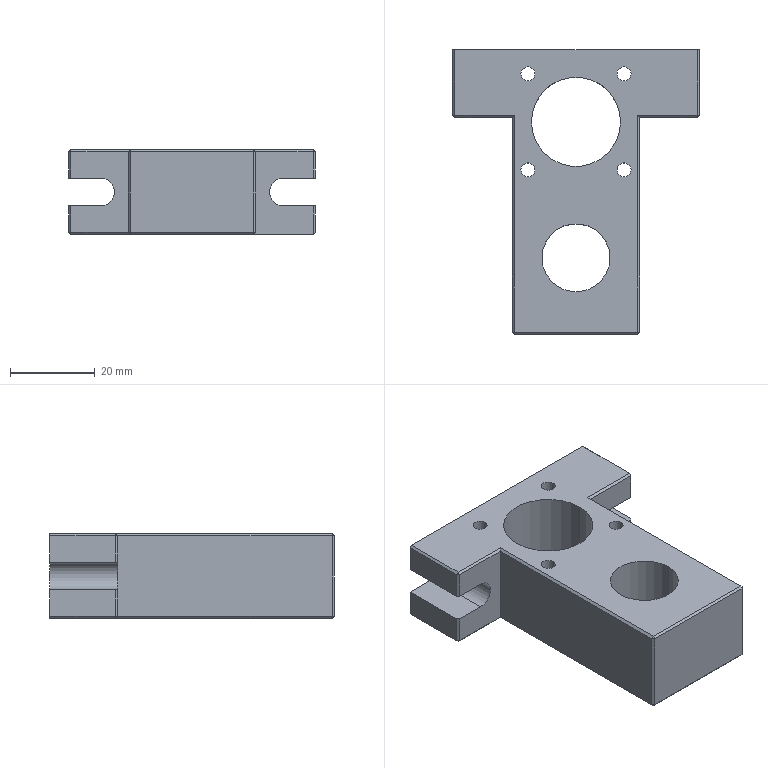Part | STEP file | 602-03-0011 | 1 solid | 56 faces | box 58 x 66.996 x 20 mm | volume 35380 mm3 | plane 42 | cylinder 14 | commonest cylinder face diameters 3.3 x8 6.5 x2 16 x2 21 x2